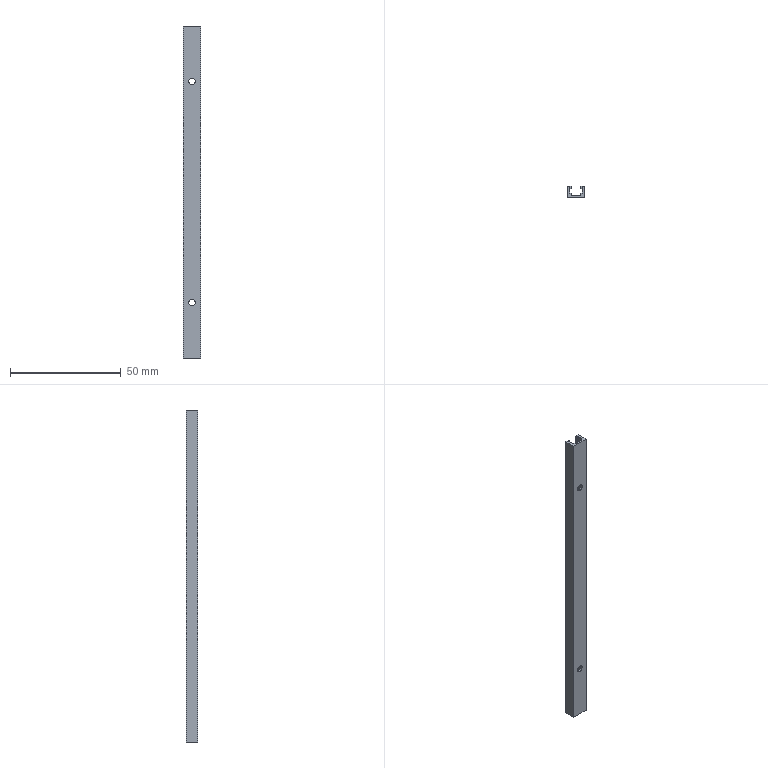Part | STEP file | module KR050 photoelectric mounting profile 150 | 1 solid | 34 faces | box 8 x 5 x 150 mm | volume 2740 mm3 | plane 18 | cylinder 16 | commonest cylinder face diameters 0.2 x12 3 x4